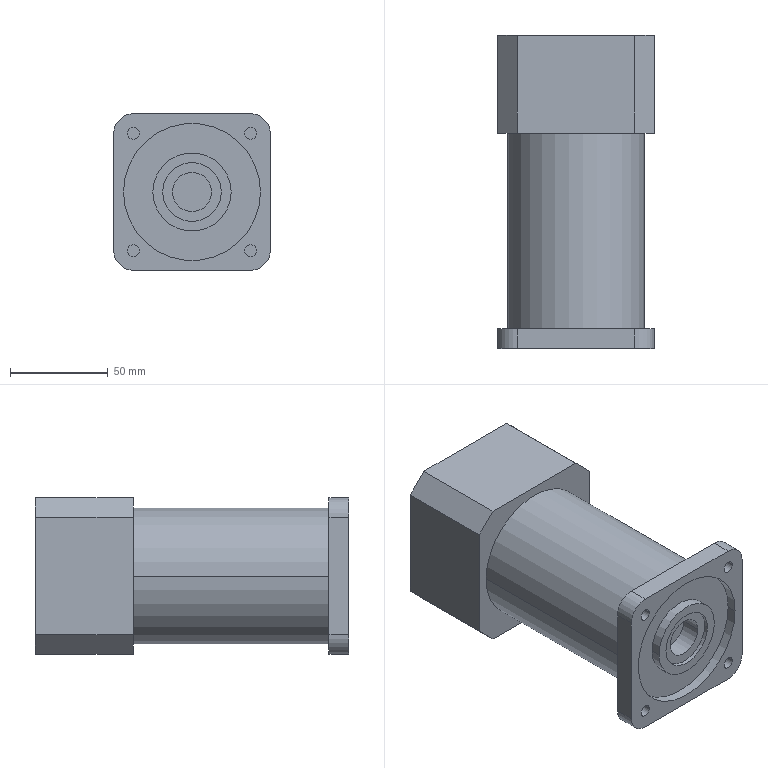Part | STEP file | Cut-Extrude 4 | 1 solid | 42 faces | box 80 x 160 x 80 mm | volume 739341 mm3 | cylinder 22 | plane 20 | commonest cylinder face diameters 6 x8 20 x6 70 x4 30 x2 40 x2
STEP:
#1=CARTESIAN_POINT('',(-1461.738,1744.264,2846.751));
#2=VERTEX_POINT('',#1);
#3=CARTESIAN_POINT('',(-1455.738,1744.264,2846.751));
#4=VERTEX_POINT('',#3);
#5=CARTESIAN_POINT('',(-1458.738,1744.264,2846.751));
#6=DIRECTION('',(0.,-1.,0.));
#7=DIRECTION('',(1.,0.,0.));
#8=AXIS2_PLACEMENT_3D('',#5,#6,#7);
#9=CIRCLE('',#8,3.);
#10=EDGE_CURVE('',#2,#4,#9,.T.);
#11=ORIENTED_EDGE('',*,*,#10,.F.);
#12=CARTESIAN_POINT('',(-1461.738,1734.264,2846.751));
#13=VERTEX_POINT('',#12);
#14=CARTESIAN_POINT('',(-1461.738,1752.264,2846.751));
#15=DIRECTION('',(0.,1.,0.));
#16=VECTOR('',#15,1000.);
#17=LINE('',#14,#16);
#18=EDGE_CURVE('',#13,#2,#17,.T.);
#19=ORIENTED_EDGE('',*,*,#18,.F.);
#20=CARTESIAN_POINT('',(-1455.738,1734.264,2846.751));
#21=VERTEX_POINT('',#20);
#22=CARTESIAN_POINT('',(-1458.738,1734.264,2846.751));
#23=DIRECTION('',(0.,-1.,0.));
#24=DIRECTION('',(-1.,0.,0.));
#25=AXIS2_PLACEMENT_3D('',#22,#23,#24);
#26=CIRCLE('',#25,3.);
#27=EDGE_CURVE('',#13,#21,#26,.T.);
#28=ORIENTED_EDGE('',*,*,#27,.T.);
#29=CARTESIAN_POINT('',(-1455.738,1752.264,2846.751));
#30=DIRECTION('',(0.,1.,0.));
#31=VECTOR('',#30,1000.);
#32=LINE('',#29,#31);
#33=EDGE_CURVE('',#21,#4,#32,.T.);
#34=ORIENTED_EDGE('',*,*,#33,.T.);
#35=EDGE_LOOP('',(#11,#19,#28,#34));
#36=FACE_OUTER_BOUND('',#35,.T.);
#37=CARTESIAN_POINT('',(-1458.738,1752.264,2846.751));
#38=DIRECTION('',(0.,-1.,0.));
#39=DIRECTION('',(-1.,0.,0.));
#40=AXIS2_PLACEMENT_3D('',#37,#38,#39);
#41=CYLINDRICAL_SURFACE('',#40,3.);
#42=ADVANCED_FACE('',(#36),#41,.F.);
#43=CARTESIAN_POINT('',(-1461.738,1744.264,2786.751));
#44=VERTEX_POINT('',#43);
#45=CARTESIAN_POINT('',(-1455.738,1744.264,2786.751));
#46=VERTEX_POINT('',#45);
#47=CARTESIAN_POINT('',(-1458.738,1744.264,2786.751));
#48=DIRECTION('',(0.,-1.,0.));
#49=DIRECTION('',(1.,0.,0.));
#50=AXIS2_PLACEMENT_3D('',#47,#48,#49);
#51=CIRCLE('',#50,3.);
#52=EDGE_CURVE('',#44,#46,#51,.T.);
#53=ORIENTED_EDGE('',*,*,#52,.F.);
#54=CARTESIAN_POINT('',(-1461.738,1734.264,2786.751));
#55=VERTEX_POINT('',#54);
#56=CARTESIAN_POINT('',(-1461.738,1752.264,2786.751));
#57=DIRECTION('',(0.,1.,0.));
#58=VECTOR('',#57,1000.);
#59=LINE('',#56,#58);
#60=EDGE_CURVE('',#55,#44,#59,.T.);
#61=ORIENTED_EDGE('',*,*,#60,.F.);
#62=CARTESIAN_POINT('',(-1455.738,1734.264,2786.751));
#63=VERTEX_POINT('',#62);
#64=CARTESIAN_POINT('',(-1458.738,1734.264,2786.751));
#65=DIRECTION('',(0.,-1.,0.));
#66=DIRECTION('',(-1.,0.,0.));
#67=AXIS2_PLACEMENT_3D('',#64,#65,#66);
#68=CIRCLE('',#67,3.);
#69=EDGE_CURVE('',#55,#63,#68,.T.);
#70=ORIENTED_EDGE('',*,*,#69,.T.);
#71=CARTESIAN_POINT('',(-1455.738,1752.264,2786.751));
#72=DIRECTION('',(0.,1.,0.));
#73=VECTOR('',#72,1000.);
#74=LINE('',#71,#73);
#75=EDGE_CURVE('',#63,#46,#74,.T.);
#76=ORIENTED_EDGE('',*,*,#75,.T.);
#77=EDGE_LOOP('',(#53,#61,#70,#76));
#78=FACE_OUTER_BOUND('',#77,.T.);
#79=CARTESIAN_POINT('',(-1458.738,1752.264,2786.751));
#80=DIRECTION('',(0.,-1.,0.));
#81=DIRECTION('',(-1.,0.,0.));
#82=AXIS2_PLACEMENT_3D('',#79,#80,#81);
#83=CYLINDRICAL_SURFACE('',#82,3.);
#84=ADVANCED_FACE('',(#78),#83,.F.);
#85=CARTESIAN_POINT('',(-1521.738,1744.264,2786.751));
#86=VERTEX_POINT('',#85);
#87=CARTESIAN_POINT('',(-1515.738,1744.264,2786.751));
#88=VERTEX_POINT('',#87);
#89=CARTESIAN_POINT('',(-1518.738,1744.264,2786.751));
#90=DIRECTION('',(0.,-1.,0.));
#91=DIRECTION('',(1.,0.,0.));
#92=AXIS2_PLACEMENT_3D('',#89,#90,#91);
#93=CIRCLE('',#92,3.);
#94=EDGE_CURVE('',#86,#88,#93,.T.);
#95=ORIENTED_EDGE('',*,*,#94,.F.);
#96=CARTESIAN_POINT('',(-1521.738,1734.264,2786.751));
#97=VERTEX_POINT('',#96);
#98=CARTESIAN_POINT('',(-1521.738,1752.264,2786.751));
#99=DIRECTION('',(0.,1.,0.));
#100=VECTOR('',#99,1000.);
#101=LINE('',#98,#100);
#102=EDGE_CURVE('',#97,#86,#101,.T.);
#103=ORIENTED_EDGE('',*,*,#102,.F.);
#104=CARTESIAN_POINT('',(-1515.738,1734.264,2786.751));
#105=VERTEX_POINT('',#104);
#106=CARTESIAN_POINT('',(-1518.738,1734.264,2786.751));
#107=DIRECTION('',(0.,-1.,0.));
#108=DIRECTION('',(1.,0.,0.));
#109=AXIS2_PLACEMENT_3D('',#106,#107,#108);
#110=CIRCLE('',#109,3.);
#111=EDGE_CURVE('',#97,#105,#110,.T.);
#112=ORIENTED_EDGE('',*,*,#111,.T.);
#113=CARTESIAN_POINT('',(-1515.738,1752.264,2786.751));
#114=DIRECTION('',(0.,1.,0.));
#115=VECTOR('',#114,1000.);
#116=LINE('',#113,#115);
#117=EDGE_CURVE('',#105,#88,#116,.T.);
#118=ORIENTED_EDGE('',*,*,#117,.T.);
#119=EDGE_LOOP('',(#95,#103,#112,#118));
#120=FACE_OUTER_BOUND('',#119,.T.);
#121=CARTESIAN_POINT('',(-1518.738,1752.264,2786.751));
#122=DIRECTION('',(0.,-1.,0.));
#123=DIRECTION('',(-1.,0.,0.));
#124=AXIS2_PLACEMENT_3D('',#121,#122,#123);
#125=CYLINDRICAL_SURFACE('',#124,3.);
#126=ADVANCED_FACE('',(#120),#125,.F.);
#127=CARTESIAN_POINT('',(-1521.738,1744.264,2846.751));
#128=VERTEX_POINT('',#127);
#129=CARTESIAN_POINT('',(-1515.738,1744.264,2846.751));
#130=VERTEX_POINT('',#129);
#131=CARTESIAN_POINT('',(-1518.738,1744.264,2846.751));
#132=DIRECTION('',(0.,-1.,0.));
#133=DIRECTION('',(1.,0.,0.));
#134=AXIS2_PLACEMENT_3D('',#131,#132,#133);
#135=CIRCLE('',#134,3.);
#136=EDGE_CURVE('',#128,#130,#135,.T.);
#137=ORIENTED_EDGE('',*,*,#136,.F.);
#138=CARTESIAN_POINT('',(-1521.738,1734.264,2846.751));
#139=VERTEX_POINT('',#138);
#140=CARTESIAN_POINT('',(-1521.738,1752.264,2846.751));
#141=DIRECTION('',(0.,1.,0.));
#142=VECTOR('',#141,1000.);
#143=LINE('',#140,#142);
#144=EDGE_CURVE('',#139,#128,#143,.T.);
#145=ORIENTED_EDGE('',*,*,#144,.F.);
#146=CARTESIAN_POINT('',(-1515.738,1734.264,2846.751));
#147=VERTEX_POINT('',#146);
#148=CARTESIAN_POINT('',(-1518.738,1734.264,2846.751));
#149=DIRECTION('',(0.,-1.,0.));
#150=DIRECTION('',(1.,0.,0.));
#151=AXIS2_PLACEMENT_3D('',#148,#149,#150);
#152=CIRCLE('',#151,3.);
#153=EDGE_CURVE('',#139,#147,#152,.T.);
#154=ORIENTED_EDGE('',*,*,#153,.T.);
#155=CARTESIAN_POINT('',(-1515.738,1752.264,2846.751));
#156=DIRECTION('',(0.,1.,0.));
#157=VECTOR('',#156,1000.);
#158=LINE('',#155,#157);
#159=EDGE_CURVE('',#147,#130,#158,.T.);
#160=ORIENTED_EDGE('',*,*,#159,.T.);
#161=EDGE_LOOP('',(#137,#145,#154,#160));
#162=FACE_OUTER_BOUND('',#161,.T.);
#163=CARTESIAN_POINT('',(-1518.738,1752.264,2846.751));
#164=DIRECTION('',(0.,-1.,0.));
#165=DIRECTION('',(-1.,0.,0.));
#166=AXIS2_PLACEMENT_3D('',#163,#164,#165);
#167=CYLINDRICAL_SURFACE('',#166,3.);
#168=ADVANCED_FACE('',(#162),#167,.F.);
#169=CARTESIAN_POINT('',(-1498.738,1746.264,2816.751));
#170=VERTEX_POINT('',#169);
#171=CARTESIAN_POINT('',(-1478.738,1746.264,2816.751));
#172=VERTEX_POINT('',#171);
#173=CARTESIAN_POINT('',(-1488.738,1746.264,2816.751));
#174=DIRECTION('',(0.,-1.,0.));
#175=DIRECTION('',(1.,0.,0.));
#176=AXIS2_PLACEMENT_3D('',#173,#174,#175);
#177=CIRCLE('',#176,10.);
#178=EDGE_CURVE('',#170,#172,#177,.T.);
#179=ORIENTED_EDGE('',*,*,#178,.F.);
#180=CARTESIAN_POINT('',(-1498.738,1736.264,2816.751));
#181=VERTEX_POINT('',#180);
#182=CARTESIAN_POINT('',(-1498.738,1746.264,2816.751));
#183=DIRECTION('',(0.,1.,0.));
#184=VECTOR('',#183,1000.);
#185=LINE('',#182,#184);
#186=EDGE_CURVE('',#181,#170,#185,.T.);
#187=ORIENTED_EDGE('',*,*,#186,.F.);
#188=CARTESIAN_POINT('',(-1478.738,1736.264,2816.751));
#189=VERTEX_POINT('',#188);
#190=CARTESIAN_POINT('',(-1488.738,1736.264,2816.751));
#191=DIRECTION('',(0.,-1.,0.));
#192=DIRECTION('',(1.,0.,0.));
#193=AXIS2_PLACEMENT_3D('',#190,#191,#192);
#194=CIRCLE('',#193,10.);
#195=EDGE_CURVE('',#181,#189,#194,.T.);
#196=ORIENTED_EDGE('',*,*,#195,.T.);
#197=CARTESIAN_POINT('',(-1478.738,1746.264,2816.751));
#198=DIRECTION('',(0.,1.,0.));
#199=VECTOR('',#198,1000.);
#200=LINE('',#197,#199);
#201=EDGE_CURVE('',#189,#172,#200,.T.);
#202=ORIENTED_EDGE('',*,*,#201,.T.);
#203=EDGE_LOOP('',(#179,#187,#196,#202));
#204=FACE_OUTER_BOUND('',#203,.T.);
#205=CARTESIAN_POINT('',(-1488.738,1746.264,2816.751));
#206=DIRECTION('',(0.,-1.,0.));
#207=DIRECTION('',(-1.,0.,0.));
#208=AXIS2_PLACEMENT_3D('',#205,#206,#207);
#209=CYLINDRICAL_SURFACE('',#208,10.);
#210=ADVANCED_FACE('',(#204),#209,.F.);
#211=CARTESIAN_POINT('',(-1503.738,1736.264,2816.751));
#212=VERTEX_POINT('',#211);
#213=CARTESIAN_POINT('',(-1473.738,1736.264,2816.751));
#214=VERTEX_POINT('',#213);
#215=CARTESIAN_POINT('',(-1488.738,1736.264,2816.751));
#216=DIRECTION('',(0.,-1.,0.));
#217=DIRECTION('',(1.,0.,0.));
#218=AXIS2_PLACEMENT_3D('',#215,#216,#217);
#219=CIRCLE('',#218,15.);
#220=EDGE_CURVE('',#212,#214,#219,.T.);
#221=ORIENTED_EDGE('',*,*,#220,.F.);
#222=CARTESIAN_POINT('',(-1503.738,1734.264,2816.751));
#223=VERTEX_POINT('',#222);
#224=CARTESIAN_POINT('',(-1503.738,1736.264,2816.751));
#225=DIRECTION('',(0.,1.,0.));
#226=VECTOR('',#225,1000.);
#227=LINE('',#224,#226);
#228=EDGE_CURVE('',#223,#212,#227,.T.);
#229=ORIENTED_EDGE('',*,*,#228,.F.);
#230=CARTESIAN_POINT('',(-1473.738,1734.264,2816.751));
#231=VERTEX_POINT('',#230);
#232=CARTESIAN_POINT('',(-1488.738,1734.264,2816.751));
#233=DIRECTION('',(0.,-1.,0.));
#234=DIRECTION('',(1.,0.,0.));
#235=AXIS2_PLACEMENT_3D('',#232,#233,#234);
#236=CIRCLE('',#235,15.);
#237=EDGE_CURVE('',#223,#231,#236,.T.);
#238=ORIENTED_EDGE('',*,*,#237,.T.);
#239=CARTESIAN_POINT('',(-1473.738,1736.264,2816.751));
#240=DIRECTION('',(0.,1.,0.));
#241=VECTOR('',#240,1000.);
#242=LINE('',#239,#241);
#243=EDGE_CURVE('',#231,#214,#242,.T.);
#244=ORIENTED_EDGE('',*,*,#243,.T.);
#245=EDGE_LOOP('',(#221,#229,#238,#244));
#246=FACE_OUTER_BOUND('',#245,.T.);
#247=CARTESIAN_POINT('',(-1488.738,1736.264,2816.751));
#248=DIRECTION('',(0.,-1.,0.));
#249=DIRECTION('',(-1.,0.,0.));
#250=AXIS2_PLACEMENT_3D('',#247,#248,#249);
#251=CYLINDRICAL_SURFACE('',#250,15.);
#252=ADVANCED_FACE('',(#246),#251,.F.);
#253=CARTESIAN_POINT('',(-1468.738,1734.264,2816.751));
#254=VERTEX_POINT('',#253);
#255=CARTESIAN_POINT('',(-1508.738,1734.264,2816.751));
#256=VERTEX_POINT('',#255);
#257=CARTESIAN_POINT('',(-1488.738,1734.264,2816.751));
#258=DIRECTION('',(0.,-1.,0.));
#259=DIRECTION('',(1.,0.,0.));
#260=AXIS2_PLACEMENT_3D('',#257,#258,#259);
#261=CIRCLE('',#260,20.);
#262=EDGE_CURVE('',#254,#256,#261,.T.);
#263=ORIENTED_EDGE('',*,*,#262,.F.);
#264=CARTESIAN_POINT('',(-1468.738,1739.264,2816.751));
#265=VERTEX_POINT('',#264);
#266=CARTESIAN_POINT('',(-1468.738,1734.264,2816.751));
#267=DIRECTION('',(0.,1.,0.));
#268=VECTOR('',#267,1000.);
#269=LINE('',#266,#268);
#270=EDGE_CURVE('',#254,#265,#269,.T.);
#271=ORIENTED_EDGE('',*,*,#270,.T.);
#272=CARTESIAN_POINT('',(-1508.738,1739.264,2816.751));
#273=VERTEX_POINT('',#272);
#274=CARTESIAN_POINT('',(-1488.738,1739.264,2816.751));
#275=DIRECTION('',(0.,-1.,0.));
#276=DIRECTION('',(1.,0.,0.));
#277=AXIS2_PLACEMENT_3D('',#274,#275,#276);
#278=CIRCLE('',#277,20.);
#279=EDGE_CURVE('',#265,#273,#278,.T.);
#280=ORIENTED_EDGE('',*,*,#279,.T.);
#281=CARTESIAN_POINT('',(-1508.738,1734.264,2816.751));
#282=DIRECTION('',(0.,1.,0.));
#283=VECTOR('',#282,1000.);
#284=LINE('',#281,#283);
#285=EDGE_CURVE('',#256,#273,#284,.T.);
#286=ORIENTED_EDGE('',*,*,#285,.F.);
#287=EDGE_LOOP('',(#263,#271,#280,#286));
#288=FACE_OUTER_BOUND('',#287,.T.);
#289=CARTESIAN_POINT('',(-1488.738,1734.264,2816.751));
#290=DIRECTION('',(0.,1.,0.));
#291=DIRECTION('',(1.,0.,0.));
#292=AXIS2_PLACEMENT_3D('',#289,#290,#291);
#293=CYLINDRICAL_SURFACE('',#292,20.);
#294=ADVANCED_FACE('',(#288),#293,.T.);
#295=CARTESIAN_POINT('',(-1523.738,1739.264,2816.751));
#296=VERTEX_POINT('',#295);
#297=CARTESIAN_POINT('',(-1453.738,1739.264,2816.751));
#298=VERTEX_POINT('',#297);
#299=CARTESIAN_POINT('',(-1488.738,1739.264,2816.751));
#300=DIRECTION('',(0.,-1.,0.));
#301=DIRECTION('',(1.,0.,0.));
#302=AXIS2_PLACEMENT_3D('',#299,#300,#301);
#303=CIRCLE('',#302,35.);
#304=EDGE_CURVE('',#296,#298,#303,.T.);
#305=ORIENTED_EDGE('',*,*,#304,.F.);
#306=CARTESIAN_POINT('',(-1523.738,1734.264,2816.751));
#307=VERTEX_POINT('',#306);
#308=CARTESIAN_POINT('',(-1523.738,1739.264,2816.751));
#309=DIRECTION('',(0.,1.,0.));
#310=VECTOR('',#309,1000.);
#311=LINE('',#308,#310);
#312=EDGE_CURVE('',#307,#296,#311,.T.);
#313=ORIENTED_EDGE('',*,*,#312,.F.);
#314=CARTESIAN_POINT('',(-1453.738,1734.264,2816.751));
#315=VERTEX_POINT('',#314);
#316=CARTESIAN_POINT('',(-1488.738,1734.264,2816.751));
#317=DIRECTION('',(0.,-1.,0.));
#318=DIRECTION('',(1.,0.,0.));
#319=AXIS2_PLACEMENT_3D('',#316,#317,#318);
#320=CIRCLE('',#319,35.);
#321=EDGE_CURVE('',#307,#315,#320,.T.);
#322=ORIENTED_EDGE('',*,*,#321,.T.);
#323=CARTESIAN_POINT('',(-1453.738,1739.264,2816.751));
#324=DIRECTION('',(0.,1.,0.));
#325=VECTOR('',#324,1000.);
#326=LINE('',#323,#325);
#327=EDGE_CURVE('',#315,#298,#326,.T.);
#328=ORIENTED_EDGE('',*,*,#327,.T.);
#329=EDGE_LOOP('',(#305,#313,#322,#328));
#330=FACE_OUTER_BOUND('',#329,.T.);
#331=CARTESIAN_POINT('',(-1488.738,1739.264,2816.751));
#332=DIRECTION('',(0.,-1.,0.));
#333=DIRECTION('',(-1.,0.,0.));
#334=AXIS2_PLACEMENT_3D('',#331,#332,#333);
#335=CYLINDRICAL_SURFACE('',#334,35.);
#336=ADVANCED_FACE('',(#330),#335,.F.);
#337=CARTESIAN_POINT('',(-1453.738,1744.264,2816.751));
#338=VERTEX_POINT('',#337);
#339=CARTESIAN_POINT('',(-1523.738,1744.264,2816.751));
#340=VERTEX_POINT('',#339);
#341=CARTESIAN_POINT('',(-1488.738,1744.264,2816.751));
#342=DIRECTION('',(0.,-1.,0.));
#343=DIRECTION('',(1.,0.,0.));
#344=AXIS2_PLACEMENT_3D('',#341,#342,#343);
#345=CIRCLE('',#344,35.);
#346=EDGE_CURVE('',#338,#340,#345,.T.);
#347=ORIENTED_EDGE('',*,*,#346,.F.);
#348=CARTESIAN_POINT('',(-1453.738,1844.264,2816.751));
#349=VERTEX_POINT('',#348);
#350=CARTESIAN_POINT('',(-1453.738,1744.264,2816.751));
#351=DIRECTION('',(0.,1.,0.));
#352=VECTOR('',#351,1000.);
#353=LINE('',#350,#352);
#354=EDGE_CURVE('',#338,#349,#353,.T.);
#355=ORIENTED_EDGE('',*,*,#354,.T.);
#356=CARTESIAN_POINT('',(-1523.738,1844.264,2816.751));
#357=VERTEX_POINT('',#356);
#358=CARTESIAN_POINT('',(-1488.738,1844.264,2816.751));
#359=DIRECTION('',(0.,-1.,0.));
#360=DIRECTION('',(-1.,0.,0.));
#361=AXIS2_PLACEMENT_3D('',#358,#359,#360);
#362=CIRCLE('',#361,35.);
#363=EDGE_CURVE('',#349,#357,#362,.T.);
#364=ORIENTED_EDGE('',*,*,#363,.T.);
#365=CARTESIAN_POINT('',(-1523.738,1744.264,2816.751));
#366=DIRECTION('',(0.,1.,0.));
#367=VECTOR('',#366,1000.);
#368=LINE('',#365,#367);
#369=EDGE_CURVE('',#340,#357,#368,.T.);
#370=ORIENTED_EDGE('',*,*,#369,.F.);
#371=EDGE_LOOP('',(#347,#355,#364,#370));
#372=FACE_OUTER_BOUND('',#371,.T.);
#373=CARTESIAN_POINT('',(-1488.738,1744.264,2816.751));
#374=DIRECTION('',(0.,1.,0.));
#375=DIRECTION('',(1.,0.,0.));
#376=AXIS2_PLACEMENT_3D('',#373,#374,#375);
#377=CYLINDRICAL_SURFACE('',#376,35.);
#378=ADVANCED_FACE('',(#372),#377,.T.);
#379=CARTESIAN_POINT('',(-1488.738,1739.264,2816.751));
#380=DIRECTION('',(0.,-1.,0.));
#381=DIRECTION('',(1.,0.,0.));
#382=AXIS2_PLACEMENT_3D('',#379,#380,#381);
#383=CIRCLE('',#382,35.);
#384=EDGE_CURVE('',#298,#296,#383,.T.);
#385=ORIENTED_EDGE('',*,*,#384,.T.);
#386=ORIENTED_EDGE('',*,*,#304,.T.);
#387=EDGE_LOOP('',(#385,#386));
#388=FACE_OUTER_BOUND('',#387,.T.);
#389=CARTESIAN_POINT('',(-1488.738,1739.264,2816.751));
#390=DIRECTION('',(0.,-1.,0.));
#391=DIRECTION('',(1.,0.,0.));
#392=AXIS2_PLACEMENT_3D('',#389,#390,#391);
#393=CIRCLE('',#392,20.);
#394=EDGE_CURVE('',#273,#265,#393,.T.);
#395=ORIENTED_EDGE('',*,*,#394,.F.);
#396=ORIENTED_EDGE('',*,*,#279,.F.);
#397=EDGE_LOOP('',(#395,#396));
#398=FACE_BOUND('',#397,.T.);
#399=CARTESIAN_POINT('',(-1488.738,1739.264,2816.751));
#400=DIRECTION('',(0.,-1.,0.));
#401=DIRECTION('',(-1.,0.,0.));
#402=AXIS2_PLACEMENT_3D('',#399,#400,#401);
#403=PLANE('',#402);
#404=ADVANCED_FACE('',(#388,#398),#403,.T.);
#405=CARTESIAN_POINT('',(-1458.738,1844.264,2856.751));
#406=VERTEX_POINT('',#405);
#407=CARTESIAN_POINT('',(-1518.738,1844.264,2856.751));
#408=VERTEX_POINT('',#407);
#409=CARTESIAN_POINT('',(-1518.738,1844.264,2856.751));
#410=DIRECTION('',(-1.,0.,0.));
#411=VECTOR('',#410,1000.);
#412=LINE('',#409,#411);
#413=EDGE_CURVE('',#406,#408,#412,.T.);
#414=ORIENTED_EDGE('',*,*,#413,.T.);
#415=CARTESIAN_POINT('',(-1528.738,1844.264,2846.751));
#416=VERTEX_POINT('',#415);
#417=CARTESIAN_POINT('',(-1528.738,1844.264,2846.751));
#418=DIRECTION('',(-0.7071,0.,-0.7071));
#419=VECTOR('',#418,1000.);
#420=LINE('',#417,#419);
#421=EDGE_CURVE('',#408,#416,#420,.T.);
#422=ORIENTED_EDGE('',*,*,#421,.T.);
#423=CARTESIAN_POINT('',(-1528.738,1844.264,2786.751));
#424=VERTEX_POINT('',#423);
#425=CARTESIAN_POINT('',(-1528.738,1844.264,2846.751));
#426=DIRECTION('',(0.,0.,-1.));
#427=VECTOR('',#426,1000.);
#428=LINE('',#425,#427);
#429=EDGE_CURVE('',#416,#424,#428,.T.);
#430=ORIENTED_EDGE('',*,*,#429,.T.);
#431=CARTESIAN_POINT('',(-1518.738,1844.264,2776.751));
#432=VERTEX_POINT('',#431);
#433=CARTESIAN_POINT('',(-1528.738,1844.264,2786.751));
#434=DIRECTION('',(0.7071,0.,-0.7071));
#435=VECTOR('',#434,1000.);
#436=LINE('',#433,#435);
#437=EDGE_CURVE('',#424,#432,#436,.T.);
#438=ORIENTED_EDGE('',*,*,#437,.T.);
#439=CARTESIAN_POINT('',(-1458.738,1844.264,2776.751));
#440=VERTEX_POINT('',#439);
#441=CARTESIAN_POINT('',(-1518.738,1844.264,2776.751));
#442=DIRECTION('',(1.,0.,0.));
#443=VECTOR('',#442,1000.);
#444=LINE('',#441,#443);
#445=EDGE_CURVE('',#432,#440,#444,.T.);
#446=ORIENTED_EDGE('',*,*,#445,.T.);
#447=CARTESIAN_POINT('',(-1448.738,1844.264,2786.751));
#448=VERTEX_POINT('',#447);
#449=CARTESIAN_POINT('',(-1458.738,1844.264,2776.751));
#450=DIRECTION('',(0.7071,0.,0.7071));
#451=VECTOR('',#450,1000.);
#452=LINE('',#449,#451);
#453=EDGE_CURVE('',#440,#448,#452,.T.);
#454=ORIENTED_EDGE('',*,*,#453,.T.);
#455=CARTESIAN_POINT('',(-1448.738,1844.264,2846.751));
#456=VERTEX_POINT('',#455);
#457=CARTESIAN_POINT('',(-1448.738,1844.264,2846.751));
#458=DIRECTION('',(0.,0.,1.));
#459=VECTOR('',#458,1000.);
#460=LINE('',#457,#459);
#461=EDGE_CURVE('',#448,#456,#460,.T.);
#462=ORIENTED_EDGE('',*,*,#461,.T.);
#463=CARTESIAN_POINT('',(-1458.738,1844.264,2856.751));
#464=DIRECTION('',(-0.7071,0.,0.7071));
#465=VECTOR('',#464,1000.);
#466=LINE('',#463,#465);
#467=EDGE_CURVE('',#456,#406,#466,.T.);
#468=ORIENTED_EDGE('',*,*,#467,.T.);
#469=EDGE_LOOP('',(#414,#422,#430,#438,#446,#454,#462,#468));
#470=FACE_OUTER_BOUND('',#469,.T.);
#471=CARTESIAN_POINT('',(-1488.738,1844.264,2816.751));
#472=DIRECTION('',(0.,-1.,0.));
#473=DIRECTION('',(-1.,0.,0.));
#474=AXIS2_PLACEMENT_3D('',#471,#472,#473);
#475=CIRCLE('',#474,35.);
#476=EDGE_CURVE('',#357,#349,#475,.T.);
#477=ORIENTED_EDGE('',*,*,#476,.F.);
#478=ORIENTED_EDGE('',*,*,#363,.F.);
#479=EDGE_LOOP('',(#477,#478));
#480=FACE_BOUND('',#479,.T.);
#481=CARTESIAN_POINT('',(-1488.738,1844.264,2816.751));
#482=DIRECTION('',(0.,1.,0.));
#483=DIRECTION('',(1.,0.,0.));
#484=AXIS2_PLACEMENT_3D('',#481,#482,#483);
#485=PLANE('',#484);
#486=ADVANCED_FACE('',(#470,#480),#485,.F.);
#487=CARTESIAN_POINT('',(-1458.738,1894.264,2856.751));
#488=VERTEX_POINT('',#487);
#489=CARTESIAN_POINT('',(-1518.738,1894.264,2856.751));
#490=VERTEX_POINT('',#489);
#491=CARTESIAN_POINT('',(-1518.738,1894.264,2856.751));
#492=DIRECTION('',(-1.,0.,0.));
#493=VECTOR('',#492,1000.);
#494=LINE('',#491,#493);
#495=EDGE_CURVE('',#488,#490,#494,.T.);
#496=ORIENTED_EDGE('',*,*,#495,.T.);
#497=CARTESIAN_POINT('',(-1518.738,1844.264,2856.751));
#498=DIRECTION('',(0.,1.,0.));
#499=VECTOR('',#498,1000.);
#500=LINE('',#497,#499);
#501=EDGE_CURVE('',#408,#490,#500,.T.);
#502=ORIENTED_EDGE('',*,*,#501,.F.);
#503=ORIENTED_EDGE('',*,*,#413,.F.);
#504=CARTESIAN_POINT('',(-1458.738,1844.264,2856.751));
#505=DIRECTION('',(0.,1.,0.));
#506=VECTOR('',#505,1000.);
#507=LINE('',#504,#506);
#508=EDGE_CURVE('',#406,#488,#507,.T.);
#509=ORIENTED_EDGE('',*,*,#508,.T.);
#510=EDGE_LOOP('',(#496,#502,#503,#509));
#511=FACE_OUTER_BOUND('',#510,.T.);
#512=CARTESIAN_POINT('',(-1518.738,1844.264,2856.751));
#513=DIRECTION('',(0.,0.,-1.));
#514=DIRECTION('',(-1.,0.,0.));
#515=AXIS2_PLACEMENT_3D('',#512,#513,#514);
#516=PLANE('',#515);
#517=ADVANCED_FACE('',(#511),#516,.F.);
#518=CARTESIAN_POINT('',(-1528.738,1894.264,2846.751));
#519=VERTEX_POINT('',#518);
#520=CARTESIAN_POINT('',(-1528.738,1894.264,2846.751));
#521=DIRECTION('',(-0.7071,0.,-0.7071));
#522=VECTOR('',#521,1000.);
#523=LINE('',#520,#522);
#524=EDGE_CURVE('',#490,#519,#523,.T.);
#525=ORIENTED_EDGE('',*,*,#524,.T.);
#526=CARTESIAN_POINT('',(-1528.738,1844.264,2846.751));
#527=DIRECTION('',(0.,1.,0.));
#528=VECTOR('',#527,1000.);
#529=LINE('',#526,#528);
#530=EDGE_CURVE('',#416,#519,#529,.T.);
#531=ORIENTED_EDGE('',*,*,#530,.F.);
#532=ORIENTED_EDGE('',*,*,#421,.F.);
#533=ORIENTED_EDGE('',*,*,#501,.T.);
#534=EDGE_LOOP('',(#525,#531,#532,#533));
#535=FACE_OUTER_BOUND('',#534,.T.);
#536=CARTESIAN_POINT('',(-1528.738,1844.264,2846.751));
#537=DIRECTION('',(0.7071,0.,-0.7071));
#538=DIRECTION('',(-0.7071,0.,-0.7071));
#539=AXIS2_PLACEMENT_3D('',#536,#537,#538);
#540=PLANE('',#539);
#541=ADVANCED_FACE('',(#535),#540,.F.);
#542=CARTESIAN_POINT('',(-1528.738,1894.264,2786.751));
#543=VERTEX_POINT('',#542);
#544=CARTESIAN_POINT('',(-1528.738,1894.264,2846.751));
#545=DIRECTION('',(0.,0.,-1.));
#546=VECTOR('',#545,1000.);
#547=LINE('',#544,#546);
#548=EDGE_CURVE('',#519,#543,#547,.T.);
#549=ORIENTED_EDGE('',*,*,#548,.T.);
#550=CARTESIAN_POINT('',(-1528.738,1844.264,2786.751));
#551=DIRECTION('',(0.,1.,0.));
#552=VECTOR('',#551,1000.);
#553=LINE('',#550,#552);
#554=EDGE_CURVE('',#424,#543,#553,.T.);
#555=ORIENTED_EDGE('',*,*,#554,.F.);
#556=ORIENTED_EDGE('',*,*,#429,.F.);
#557=ORIENTED_EDGE('',*,*,#530,.T.);
#558=EDGE_LOOP('',(#549,#555,#556,#557));
#559=FACE_OUTER_BOUND('',#558,.T.);
#560=CARTESIAN_POINT('',(-1528.738,1844.264,2846.751));
#561=DIRECTION('',(1.,0.,0.));
#562=DIRECTION('',(0.,-1.,0.));
#563=AXIS2_PLACEMENT_3D('',#560,#561,#562);
#564=PLANE('',#563);
#565=ADVANCED_FACE('',(#559),#564,.F.);
#566=CARTESIAN_POINT('',(-1518.738,1894.264,2776.751));
#567=VERTEX_POINT('',#566);
#568=CARTESIAN_POINT('',(-1528.738,1894.264,2786.751));
#569=DIRECTION('',(0.7071,0.,-0.7071));
#570=VECTOR('',#569,1000.);
#571=LINE('',#568,#570);
#572=EDGE_CURVE('',#543,#567,#571,.T.);
#573=ORIENTED_EDGE('',*,*,#572,.T.);
#574=CARTESIAN_POINT('',(-1518.738,1844.264,2776.751));
#575=DIRECTION('',(0.,1.,0.));
#576=VECTOR('',#575,1000.);
#577=LINE('',#574,#576);
#578=EDGE_CURVE('',#432,#567,#577,.T.);
#579=ORIENTED_EDGE('',*,*,#578,.F.);
#580=ORIENTED_EDGE('',*,*,#437,.F.);
#581=ORIENTED_EDGE('',*,*,#554,.T.);
#582=EDGE_LOOP('',(#573,#579,#580,#581));
#583=FACE_OUTER_BOUND('',#582,.T.);
#584=CARTESIAN_POINT('',(-1528.738,1844.264,2786.751));
#585=DIRECTION('',(0.7071,0.,0.7071));
#586=DIRECTION('',(0.7071,0.,-0.7071));
#587=AXIS2_PLACEMENT_3D('',#584,#585,#586);
#588=PLANE('',#587);
#589=ADVANCED_FACE('',(#583),#588,.F.);
#590=CARTESIAN_POINT('',(-1458.738,1894.264,2776.751));
#591=VERTEX_POINT('',#590);
#592=CARTESIAN_POINT('',(-1518.738,1894.264,2776.751));
#593=DIRECTION('',(1.,0.,0.));
#594=VECTOR('',#593,1000.);
#595=LINE('',#592,#594);
#596=EDGE_CURVE('',#567,#591,#595,.T.);
#597=ORIENTED_EDGE('',*,*,#596,.T.);
#598=CARTESIAN_POINT('',(-1458.738,1844.264,2776.751));
#599=DIRECTION('',(0.,1.,0.));
#600=VECTOR('',#599,1000.);
#601=LINE('',#598,#600);
#602=EDGE_CURVE('',#440,#591,#601,.T.);
#603=ORIENTED_EDGE('',*,*,#602,.F.);
#604=ORIENTED_EDGE('',*,*,#445,.F.);
#605=ORIENTED_EDGE('',*,*,#578,.T.);
#606=EDGE_LOOP('',(#597,#603,#604,#605));
#607=FACE_OUTER_BOUND('',#606,.T.);
#608=CARTESIAN_POINT('',(-1518.738,1844.264,2776.751));
#609=DIRECTION('',(0.,0.,1.));
#610=DIRECTION('',(1.,0.,0.));
#611=AXIS2_PLACEMENT_3D('',#608,#609,#610);
#612=PLANE('',#611);
#613=ADVANCED_FACE('',(#607),#612,.F.);
#614=CARTESIAN_POINT('',(-1448.738,1894.264,2786.751));
#615=VERTEX_POINT('',#614);
#616=CARTESIAN_POINT('',(-1458.738,1894.264,2776.751));
#617=DIRECTION('',(0.7071,0.,0.7071));
#618=VECTOR('',#617,1000.);
#619=LINE('',#616,#618);
#620=EDGE_CURVE('',#591,#615,#619,.T.);
#621=ORIENTED_EDGE('',*,*,#620,.T.);
#622=CARTESIAN_POINT('',(-1448.738,1844.264,2786.751));
#623=DIRECTION('',(0.,1.,0.));
#624=VECTOR('',#623,1000.);
#625=LINE('',#622,#624);
#626=EDGE_CURVE('',#448,#615,#625,.T.);
#627=ORIENTED_EDGE('',*,*,#626,.F.);
#628=ORIENTED_EDGE('',*,*,#453,.F.);
#629=ORIENTED_EDGE('',*,*,#602,.T.);
#630=EDGE_LOOP('',(#621,#627,#628,#629));
#631=FACE_OUTER_BOUND('',#630,.T.);
#632=CARTESIAN_POINT('',(-1458.738,1844.264,2776.751));
#633=DIRECTION('',(-0.7071,0.,0.7071));
#634=DIRECTION('',(0.7071,0.,0.7071));
#635=AXIS2_PLACEMENT_3D('',#632,#633,#634);
#636=PLANE('',#635);
#637=ADVANCED_FACE('',(#631),#636,.F.);
#638=CARTESIAN_POINT('',(-1448.738,1894.264,2846.751));
#639=VERTEX_POINT('',#638);
#640=CARTESIAN_POINT('',(-1448.738,1894.264,2846.751));
#641=DIRECTION('',(0.,0.,1.));
#642=VECTOR('',#641,1000.);
#643=LINE('',#640,#642);
#644=EDGE_CURVE('',#615,#639,#643,.T.);
#645=ORIENTED_EDGE('',*,*,#644,.T.);
#646=CARTESIAN_POINT('',(-1448.738,1844.264,2846.751));
#647=DIRECTION('',(0.,1.,0.));
#648=VECTOR('',#647,1000.);
#649=LINE('',#646,#648);
#650=EDGE_CURVE('',#456,#639,#649,.T.);
#651=ORIENTED_EDGE('',*,*,#650,.F.);
#652=ORIENTED_EDGE('',*,*,#461,.F.);
#653=ORIENTED_EDGE('',*,*,#626,.T.);
#654=EDGE_LOOP('',(#645,#651,#652,#653));
#655=FACE_OUTER_BOUND('',#654,.T.);
#656=CARTESIAN_POINT('',(-1448.738,1844.264,2846.751));
#657=DIRECTION('',(-1.,0.,0.));
#658=DIRECTION('',(0.,0.,1.));
#659=AXIS2_PLACEMENT_3D('',#656,#657,#658);
#660=PLANE('',#659);
#661=ADVANCED_FACE('',(#655),#660,.F.);
#662=CARTESIAN_POINT('',(-1458.738,1894.264,2856.751));
#663=DIRECTION('',(-0.7071,0.,0.7071));
#664=VECTOR('',#663,1000.);
#665=LINE('',#662,#664);
#666=EDGE_CURVE('',#639,#488,#665,.T.);
#667=ORIENTED_EDGE('',*,*,#666,.T.);
#668=ORIENTED_EDGE('',*,*,#508,.F.);
#669=ORIENTED_EDGE('',*,*,#467,.F.);
#670=ORIENTED_EDGE('',*,*,#650,.T.);
#671=EDGE_LOOP('',(#667,#668,#669,#670));
#672=FACE_OUTER_BOUND('',#671,.T.);
#673=CARTESIAN_POINT('',(-1458.738,1844.264,2856.751));
#674=DIRECTION('',(-0.7071,0.,-0.7071));
#675=DIRECTION('',(-0.7071,0.,0.7071));
#676=AXIS2_PLACEMENT_3D('',#673,#674,#675);
#677=PLANE('',#676);
#678=ADVANCED_FACE('',(#672),#677,.F.);
#679=ORIENTED_EDGE('',*,*,#495,.F.);
#680=ORIENTED_EDGE('',*,*,#666,.F.);
#681=ORIENTED_EDGE('',*,*,#644,.F.);
#682=ORIENTED_EDGE('',*,*,#620,.F.);
#683=ORIENTED_EDGE('',*,*,#596,.F.);
#684=ORIENTED_EDGE('',*,*,#572,.F.);
#685=ORIENTED_EDGE('',*,*,#548,.F.);
#686=ORIENTED_EDGE('',*,*,#524,.F.);
#687=EDGE_LOOP('',(#679,#680,#681,#682,#683,#684,#685,#686));
#688=FACE_OUTER_BOUND('',#687,.T.);
#689=CARTESIAN_POINT('',(-1488.738,1894.264,2816.751));
#690=DIRECTION('',(0.,1.,0.));
#691=DIRECTION('',(1.,0.,0.));
#692=AXIS2_PLACEMENT_3D('',#689,#690,#691);
#693=PLANE('',#692);
#694=ADVANCED_FACE('',(#688),#693,.T.);
#695=ORIENTED_EDGE('',*,*,#354,.F.);
#696=CARTESIAN_POINT('',(-1488.738,1744.264,2816.751));
#697=DIRECTION('',(0.,-1.,0.));
#698=DIRECTION('',(1.,0.,0.));
#699=AXIS2_PLACEMENT_3D('',#696,#697,#698);
#700=CIRCLE('',#699,35.);
#701=EDGE_CURVE('',#340,#338,#700,.T.);
#702=ORIENTED_EDGE('',*,*,#701,.F.);
#703=ORIENTED_EDGE('',*,*,#369,.T.);
#704=ORIENTED_EDGE('',*,*,#476,.T.);
#705=EDGE_LOOP('',(#695,#702,#703,#704));
#706=FACE_OUTER_BOUND('',#705,.T.);
#707=CARTESIAN_POINT('',(-1488.738,1744.264,2816.751));
#708=DIRECTION('',(0.,1.,0.));
#709=DIRECTION('',(1.,0.,0.));
#710=AXIS2_PLACEMENT_3D('',#707,#708,#709);
#711=CYLINDRICAL_SURFACE('',#710,35.);
#712=ADVANCED_FACE('',(#706),#711,.T.);
#713=CARTESIAN_POINT('',(-1458.738,1744.264,2846.751));
#714=DIRECTION('',(0.,-1.,0.));
#715=DIRECTION('',(1.,0.,0.));
#716=AXIS2_PLACEMENT_3D('',#713,#714,#715);
#717=CIRCLE('',#716,3.);
#718=EDGE_CURVE('',#4,#2,#717,.T.);
#719=ORIENTED_EDGE('',*,*,#718,.T.);
#720=ORIENTED_EDGE('',*,*,#10,.T.);
#721=EDGE_LOOP('',(#719,#720));
#722=FACE_BOUND('',#721,.T.);
#723=CARTESIAN_POINT('',(-1458.738,1744.264,2786.751));
#724=DIRECTION('',(0.,-1.,0.));
#725=DIRECTION('',(1.,0.,0.));
#726=AXIS2_PLACEMENT_3D('',#723,#724,#725);
#727=CIRCLE('',#726,3.);
#728=EDGE_CURVE('',#46,#44,#727,.T.);
#729=ORIENTED_EDGE('',*,*,#728,.T.);
#730=ORIENTED_EDGE('',*,*,#52,.T.);
#731=EDGE_LOOP('',(#729,#730));
#732=FACE_BOUND('',#731,.T.);
#733=CARTESIAN_POINT('',(-1518.738,1744.264,2786.751));
#734=DIRECTION('',(0.,-1.,0.));
#735=DIRECTION('',(1.,0.,0.));
#736=AXIS2_PLACEMENT_3D('',#733,#734,#735);
#737=CIRCLE('',#736,3.);
#738=EDGE_CURVE('',#88,#86,#737,.T.);
#739=ORIENTED_EDGE('',*,*,#738,.T.);
#740=ORIENTED_EDGE('',*,*,#94,.T.);
#741=EDGE_LOOP('',(#739,#740));
#742=FACE_BOUND('',#741,.T.);
#743=CARTESIAN_POINT('',(-1518.738,1744.264,2846.751));
#744=DIRECTION('',(0.,-1.,0.));
#745=DIRECTION('',(1.,0.,0.));
#746=AXIS2_PLACEMENT_3D('',#743,#744,#745);
#747=CIRCLE('',#746,3.);
#748=EDGE_CURVE('',#130,#128,#747,.T.);
#749=ORIENTED_EDGE('',*,*,#748,.T.);
#750=ORIENTED_EDGE('',*,*,#136,.T.);
#751=EDGE_LOOP('',(#749,#750));
#752=FACE_BOUND('',#751,.T.);
#753=CARTESIAN_POINT('',(-1518.738,1744.264,2776.751));
#754=VERTEX_POINT('',#753);
#755=CARTESIAN_POINT('',(-1458.738,1744.264,2776.751));
#756=VERTEX_POINT('',#755);
#757=CARTESIAN_POINT('',(-1528.738,1744.264,2776.751));
#758=DIRECTION('',(1.,0.,0.));
#759=VECTOR('',#758,1000.);
#760=LINE('',#757,#759);
#761=EDGE_CURVE('',#754,#756,#760,.T.);
#762=ORIENTED_EDGE('',*,*,#761,.F.);
#763=CARTESIAN_POINT('',(-1528.738,1744.264,2786.751));
#764=VERTEX_POINT('',#763);
#765=CARTESIAN_POINT('',(-1518.738,1744.264,2786.751));
#766=DIRECTION('',(0.,1.,0.));
#767=DIRECTION('',(1.,0.,0.));
#768=AXIS2_PLACEMENT_3D('',#765,#766,#767);
#769=CIRCLE('',#768,10.);
#770=EDGE_CURVE('',#754,#764,#769,.T.);
#771=ORIENTED_EDGE('',*,*,#770,.T.);
#772=CARTESIAN_POINT('',(-1528.738,1744.264,2846.751));
#773=VERTEX_POINT('',#772);
#774=CARTESIAN_POINT('',(-1528.738,1744.264,2856.751));
#775=DIRECTION('',(0.,0.,-1.));
#776=VECTOR('',#775,1000.);
#777=LINE('',#774,#776);
#778=EDGE_CURVE('',#773,#764,#777,.T.);
#779=ORIENTED_EDGE('',*,*,#778,.F.);
#780=CARTESIAN_POINT('',(-1518.738,1744.264,2856.751));
#781=VERTEX_POINT('',#780);
#782=CARTESIAN_POINT('',(-1518.738,1744.264,2846.751));
#783=DIRECTION('',(0.,1.,0.));
#784=DIRECTION('',(1.,0.,0.));
#785=AXIS2_PLACEMENT_3D('',#782,#783,#784);
#786=CIRCLE('',#785,10.);
#787=EDGE_CURVE('',#773,#781,#786,.T.);
#788=ORIENTED_EDGE('',*,*,#787,.T.);
#789=CARTESIAN_POINT('',(-1458.738,1744.264,2856.751));
#790=VERTEX_POINT('',#789);
#791=CARTESIAN_POINT('',(-1528.738,1744.264,2856.751));
#792=DIRECTION('',(-1.,0.,0.));
#793=VECTOR('',#792,1000.);
#794=LINE('',#791,#793);
#795=EDGE_CURVE('',#790,#781,#794,.T.);
#796=ORIENTED_EDGE('',*,*,#795,.F.);
#797=CARTESIAN_POINT('',(-1448.738,1744.264,2846.751));
#798=VERTEX_POINT('',#797);
#799=CARTESIAN_POINT('',(-1458.738,1744.264,2846.751));
#800=DIRECTION('',(0.,1.,0.));
#801=DIRECTION('',(1.,0.,0.));
#802=AXIS2_PLACEMENT_3D('',#799,#800,#801);
#803=CIRCLE('',#802,10.);
#804=EDGE_CURVE('',#790,#798,#803,.T.);
#805=ORIENTED_EDGE('',*,*,#804,.T.);
#806=CARTESIAN_POINT('',(-1448.738,1744.264,2786.751));
#807=VERTEX_POINT('',#806);
#808=CARTESIAN_POINT('',(-1448.738,1744.264,2856.751));
#809=DIRECTION('',(0.,0.,1.));
#810=VECTOR('',#809,1000.);
#811=LINE('',#808,#810);
#812=EDGE_CURVE('',#807,#798,#811,.T.);
#813=ORIENTED_EDGE('',*,*,#812,.F.);
#814=CARTESIAN_POINT('',(-1458.738,1744.264,2786.751));
#815=DIRECTION('',(0.,1.,0.));
#816=DIRECTION('',(1.,0.,0.));
#817=AXIS2_PLACEMENT_3D('',#814,#815,#816);
#818=CIRCLE('',#817,10.);
#819=EDGE_CURVE('',#807,#756,#818,.T.);
#820=ORIENTED_EDGE('',*,*,#819,.T.);
#821=EDGE_LOOP('',(#762,#771,#779,#788,#796,#805,#813,#820));
#822=FACE_OUTER_BOUND('',#821,.T.);
#823=ORIENTED_EDGE('',*,*,#701,.T.);
#824=ORIENTED_EDGE('',*,*,#346,.T.);
#825=EDGE_LOOP('',(#823,#824));
#826=FACE_BOUND('',#825,.T.);
#827=CARTESIAN_POINT('',(-1488.738,1744.264,2816.751));
#828=DIRECTION('',(0.,-1.,0.));
#829=DIRECTION('',(-1.,0.,0.));
#830=AXIS2_PLACEMENT_3D('',#827,#828,#829);
#831=PLANE('',#830);
#832=ADVANCED_FACE('',(#722,#732,#742,#752,#822,#826),#831,.F.);
#833=CARTESIAN_POINT('',(-1448.738,1734.264,2786.751));
#834=VERTEX_POINT('',#833);
#835=CARTESIAN_POINT('',(-1448.738,1734.264,2846.751));
#836=VERTEX_POINT('',#835);
#837=CARTESIAN_POINT('',(-1448.738,1734.264,2856.751));
#838=DIRECTION('',(0.,0.,1.));
#839=VECTOR('',#838,1000.);
#840=LINE('',#837,#839);
#841=EDGE_CURVE('',#834,#836,#840,.T.);
#842=ORIENTED_EDGE('',*,*,#841,.F.);
#843=CARTESIAN_POINT('',(-1448.738,1734.264,2786.751));
#844=DIRECTION('',(0.,1.,0.));
#845=VECTOR('',#844,1000.);
#846=LINE('',#843,#845);
#847=EDGE_CURVE('',#834,#807,#846,.T.);
#848=ORIENTED_EDGE('',*,*,#847,.T.);
#849=ORIENTED_EDGE('',*,*,#812,.T.);
#850=CARTESIAN_POINT('',(-1448.738,1734.264,2846.751));
#851=DIRECTION('',(0.,-1.,0.));
#852=VECTOR('',#851,1000.);
#853=LINE('',#850,#852);
#854=EDGE_CURVE('',#798,#836,#853,.T.);
#855=ORIENTED_EDGE('',*,*,#854,.T.);
#856=EDGE_LOOP('',(#842,#848,#849,#855));
#857=FACE_OUTER_BOUND('',#856,.T.);
#858=CARTESIAN_POINT('',(-1448.738,1734.264,2856.751));
#859=DIRECTION('',(-1.,0.,0.));
#860=DIRECTION('',(0.,0.,1.));
#861=AXIS2_PLACEMENT_3D('',#858,#859,#860);
#862=PLANE('',#861);
#863=ADVANCED_FACE('',(#857),#862,.F.);
#864=CARTESIAN_POINT('',(-1458.738,1734.264,2856.751));
#865=VERTEX_POINT('',#864);
#866=CARTESIAN_POINT('',(-1518.738,1734.264,2856.751));
#867=VERTEX_POINT('',#866);
#868=CARTESIAN_POINT('',(-1528.738,1734.264,2856.751));
#869=DIRECTION('',(-1.,0.,0.));
#870=VECTOR('',#869,1000.);
#871=LINE('',#868,#870);
#872=EDGE_CURVE('',#865,#867,#871,.T.);
#873=ORIENTED_EDGE('',*,*,#872,.F.);
#874=CARTESIAN_POINT('',(-1458.738,1734.264,2856.751));
#875=DIRECTION('',(0.,1.,0.));
#876=VECTOR('',#875,1000.);
#877=LINE('',#874,#876);
#878=EDGE_CURVE('',#865,#790,#877,.T.);
#879=ORIENTED_EDGE('',*,*,#878,.T.);
#880=ORIENTED_EDGE('',*,*,#795,.T.);
#881=CARTESIAN_POINT('',(-1518.738,1734.264,2856.751));
#882=DIRECTION('',(0.,-1.,0.));
#883=VECTOR('',#882,1000.);
#884=LINE('',#881,#883);
#885=EDGE_CURVE('',#781,#867,#884,.T.);
#886=ORIENTED_EDGE('',*,*,#885,.T.);
#887=EDGE_LOOP('',(#873,#879,#880,#886));
#888=FACE_OUTER_BOUND('',#887,.T.);
#889=CARTESIAN_POINT('',(-1528.738,1734.264,2856.751));
#890=DIRECTION('',(0.,0.,-1.));
#891=DIRECTION('',(-1.,0.,0.));
#892=AXIS2_PLACEMENT_3D('',#889,#890,#891);
#893=PLANE('',#892);
#894=ADVANCED_FACE('',(#888),#893,.F.);
#895=ORIENTED_EDGE('',*,*,#778,.T.);
#896=CARTESIAN_POINT('',(-1528.738,1734.264,2786.751));
#897=VERTEX_POINT('',#896);
#898=CARTESIAN_POINT('',(-1528.738,1734.264,2786.751));
#899=DIRECTION('',(0.,-1.,0.));
#900=VECTOR('',#899,1000.);
#901=LINE('',#898,#900);
#902=EDGE_CURVE('',#764,#897,#901,.T.);
#903=ORIENTED_EDGE('',*,*,#902,.T.);
#904=CARTESIAN_POINT('',(-1528.738,1734.264,2846.751));
#905=VERTEX_POINT('',#904);
#906=CARTESIAN_POINT('',(-1528.738,1734.264,2856.751));
#907=DIRECTION('',(0.,0.,-1.));
#908=VECTOR('',#907,1000.);
#909=LINE('',#906,#908);
#910=EDGE_CURVE('',#905,#897,#909,.T.);
#911=ORIENTED_EDGE('',*,*,#910,.F.);
#912=CARTESIAN_POINT('',(-1528.738,1734.264,2846.751));
#913=DIRECTION('',(0.,1.,0.));
#914=VECTOR('',#913,1000.);
#915=LINE('',#912,#914);
#916=EDGE_CURVE('',#905,#773,#915,.T.);
#917=ORIENTED_EDGE('',*,*,#916,.T.);
#918=EDGE_LOOP('',(#895,#903,#911,#917));
#919=FACE_OUTER_BOUND('',#918,.T.);
#920=CARTESIAN_POINT('',(-1528.738,1734.264,2856.751));
#921=DIRECTION('',(1.,0.,0.));
#922=DIRECTION('',(0.,0.,-1.));
#923=AXIS2_PLACEMENT_3D('',#920,#921,#922);
#924=PLANE('',#923);
#925=ADVANCED_FACE('',(#919),#924,.F.);
#926=CARTESIAN_POINT('',(-1518.738,1734.264,2776.751));
#927=VERTEX_POINT('',#926);
#928=CARTESIAN_POINT('',(-1458.738,1734.264,2776.751));
#929=VERTEX_POINT('',#928);
#930=CARTESIAN_POINT('',(-1528.738,1734.264,2776.751));
#931=DIRECTION('',(1.,0.,0.));
#932=VECTOR('',#931,1000.);
#933=LINE('',#930,#932);
#934=EDGE_CURVE('',#927,#929,#933,.T.);
#935=ORIENTED_EDGE('',*,*,#934,.F.);
#936=CARTESIAN_POINT('',(-1518.738,1734.264,2776.751));
#937=DIRECTION('',(0.,1.,0.));
#938=VECTOR('',#937,1000.);
#939=LINE('',#936,#938);
#940=EDGE_CURVE('',#927,#754,#939,.T.);
#941=ORIENTED_EDGE('',*,*,#940,.T.);
#942=ORIENTED_EDGE('',*,*,#761,.T.);
#943=CARTESIAN_POINT('',(-1458.738,1734.264,2776.751));
#944=DIRECTION('',(0.,-1.,0.));
#945=VECTOR('',#944,1000.);
#946=LINE('',#943,#945);
#947=EDGE_CURVE('',#756,#929,#946,.T.);
#948=ORIENTED_EDGE('',*,*,#947,.T.);
#949=EDGE_LOOP('',(#935,#941,#942,#948));
#950=FACE_OUTER_BOUND('',#949,.T.);
#951=CARTESIAN_POINT('',(-1528.738,1734.264,2776.751));
#952=DIRECTION('',(0.,0.,1.));
#953=DIRECTION('',(1.,0.,0.));
#954=AXIS2_PLACEMENT_3D('',#951,#952,#953);
#955=PLANE('',#954);
#956=ADVANCED_FACE('',(#950),#955,.F.);
#957=CARTESIAN_POINT('',(-1458.738,1734.264,2846.751));
#958=DIRECTION('',(0.,-1.,0.));
#959=DIRECTION('',(-1.,0.,0.));
#960=AXIS2_PLACEMENT_3D('',#957,#958,#959);
#961=CIRCLE('',#960,3.);
#962=EDGE_CURVE('',#21,#13,#961,.T.);
#963=ORIENTED_EDGE('',*,*,#962,.F.);
#964=ORIENTED_EDGE('',*,*,#27,.F.);
#965=EDGE_LOOP('',(#963,#964));
#966=FACE_BOUND('',#965,.T.);
#967=CARTESIAN_POINT('',(-1458.738,1734.264,2786.751));
#968=DIRECTION('',(0.,-1.,0.));
#969=DIRECTION('',(-1.,0.,0.));
#970=AXIS2_PLACEMENT_3D('',#967,#968,#969);
#971=CIRCLE('',#970,3.);
#972=EDGE_CURVE('',#63,#55,#971,.T.);
#973=ORIENTED_EDGE('',*,*,#972,.F.);
#974=ORIENTED_EDGE('',*,*,#69,.F.);
#975=EDGE_LOOP('',(#973,#974));
#976=FACE_BOUND('',#975,.T.);
#977=CARTESIAN_POINT('',(-1518.738,1734.264,2786.751));
#978=DIRECTION('',(0.,-1.,0.));
#979=DIRECTION('',(1.,0.,0.));
#980=AXIS2_PLACEMENT_3D('',#977,#978,#979);
#981=CIRCLE('',#980,3.);
#982=EDGE_CURVE('',#105,#97,#981,.T.);
#983=ORIENTED_EDGE('',*,*,#982,.F.);
#984=ORIENTED_EDGE('',*,*,#111,.F.);
#985=EDGE_LOOP('',(#983,#984));
#986=FACE_BOUND('',#985,.T.);
#987=CARTESIAN_POINT('',(-1518.738,1734.264,2846.751));
#988=DIRECTION('',(0.,-1.,0.));
#989=DIRECTION('',(1.,0.,0.));
#990=AXIS2_PLACEMENT_3D('',#987,#988,#989);
#991=CIRCLE('',#990,3.);
#992=EDGE_CURVE('',#147,#139,#991,.T.);
#993=ORIENTED_EDGE('',*,*,#992,.F.);
#994=ORIENTED_EDGE('',*,*,#153,.F.);
#995=EDGE_LOOP('',(#993,#994));
#996=FACE_BOUND('',#995,.T.);
#997=CARTESIAN_POINT('',(-1488.738,1734.264,2816.751));
#998=DIRECTION('',(0.,-1.,0.));
#999=DIRECTION('',(1.,0.,0.));
#1000=AXIS2_PLACEMENT_3D('',#997,#998,#999);
#1001=CIRCLE('',#1000,35.);
#1002=EDGE_CURVE('',#315,#307,#1001,.T.);
#1003=ORIENTED_EDGE('',*,*,#1002,.F.);
#1004=ORIENTED_EDGE('',*,*,#321,.F.);
#1005=EDGE_LOOP('',(#1003,#1004));
#1006=FACE_BOUND('',#1005,.T.);
#1007=ORIENTED_EDGE('',*,*,#910,.T.);
#1008=CARTESIAN_POINT('',(-1518.738,1734.264,2786.751));
#1009=DIRECTION('',(0.,-1.,0.));
#1010=DIRECTION('',(1.,0.,0.));
#1011=AXIS2_PLACEMENT_3D('',#1008,#1009,#1010);
#1012=CIRCLE('',#1011,10.);
#1013=EDGE_CURVE('',#897,#927,#1012,.T.);
#1014=ORIENTED_EDGE('',*,*,#1013,.T.);
#1015=ORIENTED_EDGE('',*,*,#934,.T.);
#1016=CARTESIAN_POINT('',(-1458.738,1734.264,2786.751));
#1017=DIRECTION('',(0.,-1.,0.));
#1018=DIRECTION('',(1.,0.,0.));
#1019=AXIS2_PLACEMENT_3D('',#1016,#1017,#1018);
#1020=CIRCLE('',#1019,10.);
#1021=EDGE_CURVE('',#929,#834,#1020,.T.);
#1022=ORIENTED_EDGE('',*,*,#1021,.T.);
#1023=ORIENTED_EDGE('',*,*,#841,.T.);
#1024=CARTESIAN_POINT('',(-1458.738,1734.264,2846.751));
#1025=DIRECTION('',(0.,-1.,0.));
#1026=DIRECTION('',(1.,0.,0.));
#1027=AXIS2_PLACEMENT_3D('',#1024,#1025,#1026);
#1028=CIRCLE('',#1027,10.);
#1029=EDGE_CURVE('',#836,#865,#1028,.T.);
#1030=ORIENTED_EDGE('',*,*,#1029,.T.);
#1031=ORIENTED_EDGE('',*,*,#872,.T.);
#1032=CARTESIAN_POINT('',(-1518.738,1734.264,2846.751));
#1033=DIRECTION('',(0.,-1.,0.));
#1034=DIRECTION('',(1.,0.,0.));
#1035=AXIS2_PLACEMENT_3D('',#1032,#1033,#1034);
#1036=CIRCLE('',#1035,10.);
#1037=EDGE_CURVE('',#867,#905,#1036,.T.);
#1038=ORIENTED_EDGE('',*,*,#1037,.T.);
#1039=EDGE_LOOP('',(#1007,#1014,#1015,#1022,#1023,#1030,#1031,#1038));
#1040=FACE_OUTER_BOUND('',#1039,.T.);
#1041=CARTESIAN_POINT('',(-1488.738,1734.264,2816.751));
#1042=DIRECTION('',(0.,-1.,0.));
#1043=DIRECTION('',(-1.,0.,0.));
#1044=AXIS2_PLACEMENT_3D('',#1041,#1042,#1043);
#1045=PLANE('',#1044);
#1046=ADVANCED_FACE('',(#966,#976,#986,#996,#1006,#1040),#1045,.T.);
#1047=ORIENTED_EDGE('',*,*,#312,.T.);
#1048=ORIENTED_EDGE('',*,*,#384,.F.);
#1049=ORIENTED_EDGE('',*,*,#327,.F.);
#1050=ORIENTED_EDGE('',*,*,#1002,.T.);
#1051=EDGE_LOOP('',(#1047,#1048,#1049,#1050));
#1052=FACE_OUTER_BOUND('',#1051,.T.);
#1053=CARTESIAN_POINT('',(-1488.738,1739.264,2816.751));
#1054=DIRECTION('',(0.,-1.,0.));
#1055=DIRECTION('',(-1.,0.,0.));
#1056=AXIS2_PLACEMENT_3D('',#1053,#1054,#1055);
#1057=CYLINDRICAL_SURFACE('',#1056,35.);
#1058=ADVANCED_FACE('',(#1052),#1057,.F.);
#1059=ORIENTED_EDGE('',*,*,#270,.F.);
#1060=CARTESIAN_POINT('',(-1488.738,1734.264,2816.751));
#1061=DIRECTION('',(0.,-1.,0.));
#1062=DIRECTION('',(1.,0.,0.));
#1063=AXIS2_PLACEMENT_3D('',#1060,#1061,#1062);
#1064=CIRCLE('',#1063,20.);
#1065=EDGE_CURVE('',#256,#254,#1064,.T.);
#1066=ORIENTED_EDGE('',*,*,#1065,.F.);
#1067=ORIENTED_EDGE('',*,*,#285,.T.);
#1068=ORIENTED_EDGE('',*,*,#394,.T.);
#1069=EDGE_LOOP('',(#1059,#1066,#1067,#1068));
#1070=FACE_OUTER_BOUND('',#1069,.T.);
#1071=CARTESIAN_POINT('',(-1488.738,1734.264,2816.751));
#1072=DIRECTION('',(0.,1.,0.));
#1073=DIRECTION('',(1.,0.,0.));
#1074=AXIS2_PLACEMENT_3D('',#1071,#1072,#1073);
#1075=CYLINDRICAL_SURFACE('',#1074,20.);
#1076=ADVANCED_FACE('',(#1070),#1075,.T.);
#1077=CARTESIAN_POINT('',(-1488.738,1734.264,2816.751));
#1078=DIRECTION('',(0.,-1.,0.));
#1079=DIRECTION('',(1.,0.,0.));
#1080=AXIS2_PLACEMENT_3D('',#1077,#1078,#1079);
#1081=CIRCLE('',#1080,15.);
#1082=EDGE_CURVE('',#231,#223,#1081,.T.);
#1083=ORIENTED_EDGE('',*,*,#1082,.F.);
#1084=ORIENTED_EDGE('',*,*,#237,.F.);
#1085=EDGE_LOOP('',(#1083,#1084));
#1086=FACE_BOUND('',#1085,.T.);
#1087=ORIENTED_EDGE('',*,*,#1065,.T.);
#1088=ORIENTED_EDGE('',*,*,#262,.T.);
#1089=EDGE_LOOP('',(#1087,#1088));
#1090=FACE_OUTER_BOUND('',#1089,.T.);
#1091=CARTESIAN_POINT('',(-1488.738,1734.264,2816.751));
#1092=DIRECTION('',(0.,-1.,0.));
#1093=DIRECTION('',(-1.,0.,0.));
#1094=AXIS2_PLACEMENT_3D('',#1091,#1092,#1093);
#1095=PLANE('',#1094);
#1096=ADVANCED_FACE('',(#1086,#1090),#1095,.T.);
#1097=ORIENTED_EDGE('',*,*,#228,.T.);
#1098=CARTESIAN_POINT('',(-1488.738,1736.264,2816.751));
#1099=DIRECTION('',(0.,-1.,0.));
#1100=DIRECTION('',(1.,0.,0.));
#1101=AXIS2_PLACEMENT_3D('',#1098,#1099,#1100);
#1102=CIRCLE('',#1101,15.);
#1103=EDGE_CURVE('',#214,#212,#1102,.T.);
#1104=ORIENTED_EDGE('',*,*,#1103,.F.);
#1105=ORIENTED_EDGE('',*,*,#243,.F.);
#1106=ORIENTED_EDGE('',*,*,#1082,.T.);
#1107=EDGE_LOOP('',(#1097,#1104,#1105,#1106));
#1108=FACE_OUTER_BOUND('',#1107,.T.);
#1109=CARTESIAN_POINT('',(-1488.738,1736.264,2816.751));
#1110=DIRECTION('',(0.,-1.,0.));
#1111=DIRECTION('',(-1.,0.,0.));
#1112=AXIS2_PLACEMENT_3D('',#1109,#1110,#1111);
#1113=CYLINDRICAL_SURFACE('',#1112,15.);
#1114=ADVANCED_FACE('',(#1108),#1113,.F.);
#1115=CARTESIAN_POINT('',(-1488.738,1736.264,2816.751));
#1116=DIRECTION('',(0.,-1.,0.));
#1117=DIRECTION('',(1.,0.,0.));
#1118=AXIS2_PLACEMENT_3D('',#1115,#1116,#1117);
#1119=CIRCLE('',#1118,10.);
#1120=EDGE_CURVE('',#189,#181,#1119,.T.);
#1121=ORIENTED_EDGE('',*,*,#1120,.F.);
#1122=ORIENTED_EDGE('',*,*,#195,.F.);
#1123=EDGE_LOOP('',(#1121,#1122));
#1124=FACE_BOUND('',#1123,.T.);
#1125=ORIENTED_EDGE('',*,*,#1103,.T.);
#1126=ORIENTED_EDGE('',*,*,#220,.T.);
#1127=EDGE_LOOP('',(#1125,#1126));
#1128=FACE_OUTER_BOUND('',#1127,.T.);
#1129=CARTESIAN_POINT('',(-1488.738,1736.264,2816.751));
#1130=DIRECTION('',(0.,-1.,0.));
#1131=DIRECTION('',(-1.,0.,0.));
#1132=AXIS2_PLACEMENT_3D('',#1129,#1130,#1131);
#1133=PLANE('',#1132);
#1134=ADVANCED_FACE('',(#1124,#1128),#1133,.T.);
#1135=ORIENTED_EDGE('',*,*,#1013,.F.);
#1136=ORIENTED_EDGE('',*,*,#902,.F.);
#1137=ORIENTED_EDGE('',*,*,#770,.F.);
#1138=ORIENTED_EDGE('',*,*,#940,.F.);
#1139=EDGE_LOOP('',(#1135,#1136,#1137,#1138));
#1140=FACE_OUTER_BOUND('',#1139,.T.);
#1141=CARTESIAN_POINT('',(-1518.738,1734.264,2786.751));
#1142=DIRECTION('',(0.,1.,0.));
#1143=DIRECTION('',(1.,0.,0.));
#1144=AXIS2_PLACEMENT_3D('',#1141,#1142,#1143);
#1145=CYLINDRICAL_SURFACE('',#1144,10.);
#1146=ADVANCED_FACE('',(#1140),#1145,.T.);
#1147=ORIENTED_EDGE('',*,*,#1021,.F.);
#1148=ORIENTED_EDGE('',*,*,#947,.F.);
#1149=ORIENTED_EDGE('',*,*,#819,.F.);
#1150=ORIENTED_EDGE('',*,*,#847,.F.);
#1151=EDGE_LOOP('',(#1147,#1148,#1149,#1150));
#1152=FACE_OUTER_BOUND('',#1151,.T.);
#1153=CARTESIAN_POINT('',(-1458.738,1734.264,2786.751));
#1154=DIRECTION('',(0.,1.,0.));
#1155=DIRECTION('',(1.,0.,0.));
#1156=AXIS2_PLACEMENT_3D('',#1153,#1154,#1155);
#1157=CYLINDRICAL_SURFACE('',#1156,10.);
#1158=ADVANCED_FACE('',(#1152),#1157,.T.);
#1159=ORIENTED_EDGE('',*,*,#1029,.F.);
#1160=ORIENTED_EDGE('',*,*,#854,.F.);
#1161=ORIENTED_EDGE('',*,*,#804,.F.);
#1162=ORIENTED_EDGE('',*,*,#878,.F.);
#1163=EDGE_LOOP('',(#1159,#1160,#1161,#1162));
#1164=FACE_OUTER_BOUND('',#1163,.T.);
#1165=CARTESIAN_POINT('',(-1458.738,1734.264,2846.751));
#1166=DIRECTION('',(0.,1.,0.));
#1167=DIRECTION('',(1.,0.,0.));
#1168=AXIS2_PLACEMENT_3D('',#1165,#1166,#1167);
#1169=CYLINDRICAL_SURFACE('',#1168,10.);
#1170=ADVANCED_FACE('',(#1164),#1169,.T.);
#1171=ORIENTED_EDGE('',*,*,#1037,.F.);
#1172=ORIENTED_EDGE('',*,*,#885,.F.);
#1173=ORIENTED_EDGE('',*,*,#787,.F.);
#1174=ORIENTED_EDGE('',*,*,#916,.F.);
#1175=EDGE_LOOP('',(#1171,#1172,#1173,#1174));
#1176=FACE_OUTER_BOUND('',#1175,.T.);
#1177=CARTESIAN_POINT('',(-1518.738,1734.264,2846.751));
#1178=DIRECTION('',(0.,1.,0.));
#1179=DIRECTION('',(1.,0.,0.));
#1180=AXIS2_PLACEMENT_3D('',#1177,#1178,#1179);
#1181=CYLINDRICAL_SURFACE('',#1180,10.);
#1182=ADVANCED_FACE('',(#1176),#1181,.T.);
#1183=ORIENTED_EDGE('',*,*,#186,.T.);
#1184=CARTESIAN_POINT('',(-1488.738,1746.264,2816.751));
#1185=DIRECTION('',(0.,-1.,0.));
#1186=DIRECTION('',(1.,0.,0.));
#1187=AXIS2_PLACEMENT_3D('',#1184,#1185,#1186);
#1188=CIRCLE('',#1187,10.);
#1189=EDGE_CURVE('',#172,#170,#1188,.T.);
#1190=ORIENTED_EDGE('',*,*,#1189,.F.);
#1191=ORIENTED_EDGE('',*,*,#201,.F.);
#1192=ORIENTED_EDGE('',*,*,#1120,.T.);
#1193=EDGE_LOOP('',(#1183,#1190,#1191,#1192));
#1194=FACE_OUTER_BOUND('',#1193,.T.);
#1195=CARTESIAN_POINT('',(-1488.738,1746.264,2816.751));
#1196=DIRECTION('',(0.,-1.,0.));
#1197=DIRECTION('',(-1.,0.,0.));
#1198=AXIS2_PLACEMENT_3D('',#1195,#1196,#1197);
#1199=CYLINDRICAL_SURFACE('',#1198,10.);
#1200=ADVANCED_FACE('',(#1194),#1199,.F.);
#1201=ORIENTED_EDGE('',*,*,#1189,.T.);
#1202=ORIENTED_EDGE('',*,*,#178,.T.);
#1203=EDGE_LOOP('',(#1201,#1202));
#1204=FACE_OUTER_BOUND('',#1203,.T.);
#1205=CARTESIAN_POINT('',(-1488.738,1746.264,2816.751));
#1206=DIRECTION('',(0.,-1.,0.));
#1207=DIRECTION('',(-1.,0.,0.));
#1208=AXIS2_PLACEMENT_3D('',#1205,#1206,#1207);
#1209=PLANE('',#1208);
#1210=ADVANCED_FACE('',(#1204),#1209,.T.);
#1211=ORIENTED_EDGE('',*,*,#144,.T.);
#1212=ORIENTED_EDGE('',*,*,#748,.F.);
#1213=ORIENTED_EDGE('',*,*,#159,.F.);
#1214=ORIENTED_EDGE('',*,*,#992,.T.);
#1215=EDGE_LOOP('',(#1211,#1212,#1213,#1214));
#1216=FACE_OUTER_BOUND('',#1215,.T.);
#1217=CARTESIAN_POINT('',(-1518.738,1752.264,2846.751));
#1218=DIRECTION('',(0.,-1.,0.));
#1219=DIRECTION('',(-1.,0.,0.));
#1220=AXIS2_PLACEMENT_3D('',#1217,#1218,#1219);
#1221=CYLINDRICAL_SURFACE('',#1220,3.);
#1222=ADVANCED_FACE('',(#1216),#1221,.F.);
#1223=ORIENTED_EDGE('',*,*,#102,.T.);
#1224=ORIENTED_EDGE('',*,*,#738,.F.);
#1225=ORIENTED_EDGE('',*,*,#117,.F.);
#1226=ORIENTED_EDGE('',*,*,#982,.T.);
#1227=EDGE_LOOP('',(#1223,#1224,#1225,#1226));
#1228=FACE_OUTER_BOUND('',#1227,.T.);
#1229=CARTESIAN_POINT('',(-1518.738,1752.264,2786.751));
#1230=DIRECTION('',(0.,-1.,0.));
#1231=DIRECTION('',(-1.,0.,0.));
#1232=AXIS2_PLACEMENT_3D('',#1229,#1230,#1231);
#1233=CYLINDRICAL_SURFACE('',#1232,3.);
#1234=ADVANCED_FACE('',(#1228),#1233,.F.);
#1235=ORIENTED_EDGE('',*,*,#60,.T.);
#1236=ORIENTED_EDGE('',*,*,#728,.F.);
#1237=ORIENTED_EDGE('',*,*,#75,.F.);
#1238=ORIENTED_EDGE('',*,*,#972,.T.);
#1239=EDGE_LOOP('',(#1235,#1236,#1237,#1238));
#1240=FACE_OUTER_BOUND('',#1239,.T.);
#1241=CARTESIAN_POINT('',(-1458.738,1752.264,2786.751));
#1242=DIRECTION('',(0.,-1.,0.));
#1243=DIRECTION('',(-1.,0.,0.));
#1244=AXIS2_PLACEMENT_3D('',#1241,#1242,#1243);
#1245=CYLINDRICAL_SURFACE('',#1244,3.);
#1246=ADVANCED_FACE('',(#1240),#1245,.F.);
#1247=ORIENTED_EDGE('',*,*,#18,.T.);
#1248=ORIENTED_EDGE('',*,*,#718,.F.);
#1249=ORIENTED_EDGE('',*,*,#33,.F.);
#1250=ORIENTED_EDGE('',*,*,#962,.T.);
#1251=EDGE_LOOP('',(#1247,#1248,#1249,#1250));
#1252=FACE_OUTER_BOUND('',#1251,.T.);
#1253=CARTESIAN_POINT('',(-1458.738,1752.264,2846.751));
#1254=DIRECTION('',(0.,-1.,0.));
#1255=DIRECTION('',(-1.,0.,0.));
#1256=AXIS2_PLACEMENT_3D('',#1253,#1254,#1255);
#1257=CYLINDRICAL_SURFACE('',#1256,3.);
#1258=ADVANCED_FACE('',(#1252),#1257,.F.);
#1259=CLOSED_SHELL('',(#42,#84,#126,#168,#210,#252,#294,#336,#378,#404,#486,#517,#541,#565,#589,#613,#637,#661,#678,#694,#712,#832,#863,#894,#925,#956,#1046,#1058,#1076,#1096,#1114,#1134,#1146,#1158,#1170,#1182,#1200,#1210,#1222,#1234,#1246,#1258));
#1260=MANIFOLD_SOLID_BREP('',#1259);
#1261=CARTESIAN_POINT('',(0.,0.,0.));
#1262=DIRECTION('',(0.,0.,1.));
#1263=DIRECTION('',(1.,0.,0.));
#1264=AXIS2_PLACEMENT_3D('',#1261,#1262,#1263);
#1265=(LENGTH_UNIT()NAMED_UNIT(*)SI_UNIT(.MILLI.,.METRE.));
#1266=UNCERTAINTY_MEASURE_WITH_UNIT(LENGTH_MEASURE(0.00001),#1265,'','');
#1267=(NAMED_UNIT(*)PLANE_ANGLE_UNIT()SI_UNIT($,.RADIAN.));
#1268=(NAMED_UNIT(*)SI_UNIT($,.STERADIAN.)SOLID_ANGLE_UNIT());
#1269=(GEOMETRIC_REPRESENTATION_CONTEXT(3)GLOBAL_UNCERTAINTY_ASSIGNED_CONTEXT((#1266))GLOBAL_UNIT_ASSIGNED_CONTEXT((#1265,#1267,#1268))REPRESENTATION_CONTEXT('',''));
#1270=ADVANCED_BREP_SHAPE_REPRESENTATION('',(#1260,#1264),#1269);